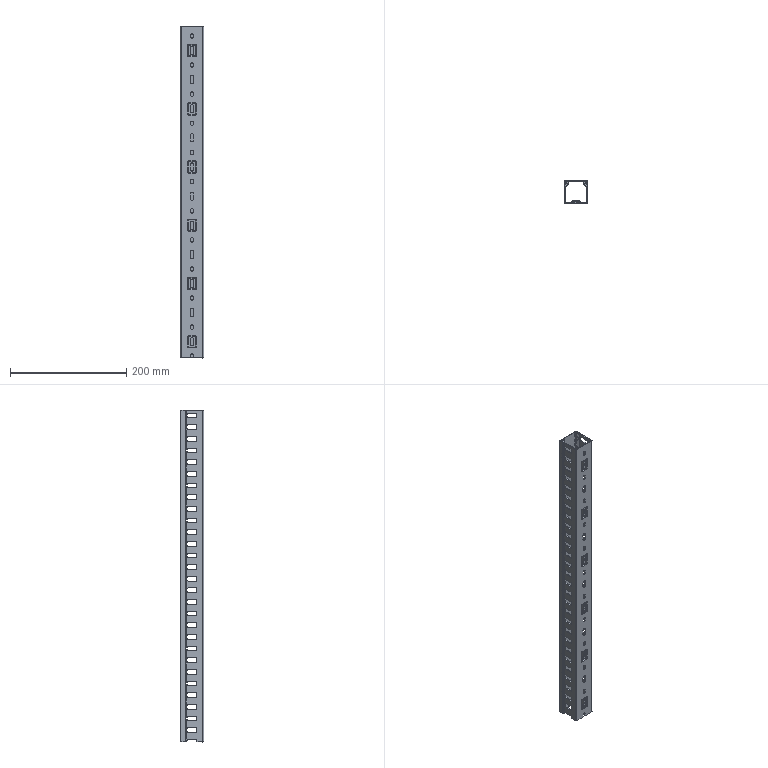Part | SolidWorks | features BaseBody 2 | 2 solids | 2174 faces | box 40 x 40.1 x 570 mm | volume 156325 mm3 | cylinder 1195 | plane 835 | sphere 96 | torus 48 | commonest cylinder face diameters 4 x228 1 x182 3 x174 3.6 x174 1.464 x144 1.4 x116